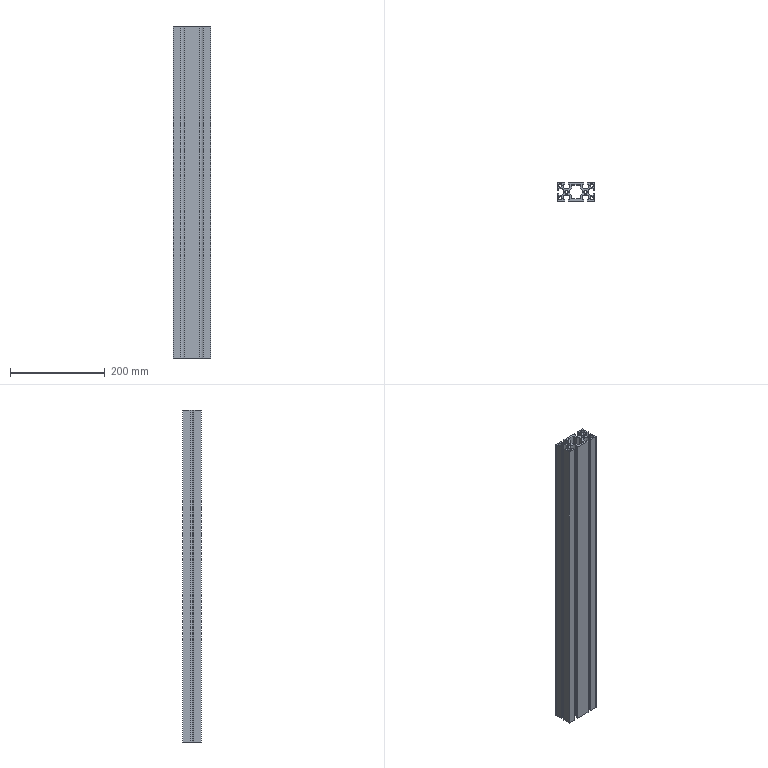Part | STEP file | 40x80 aluminium profile (L=700) | 1 solid | 87 faces | box 80 x 40 x 700 mm | volume 933883 mm3 | plane 60 | cylinder 27 | commonest cylinder face diameters 8 x8 17.549 x7 1 x4 4 x4 6.8 x4